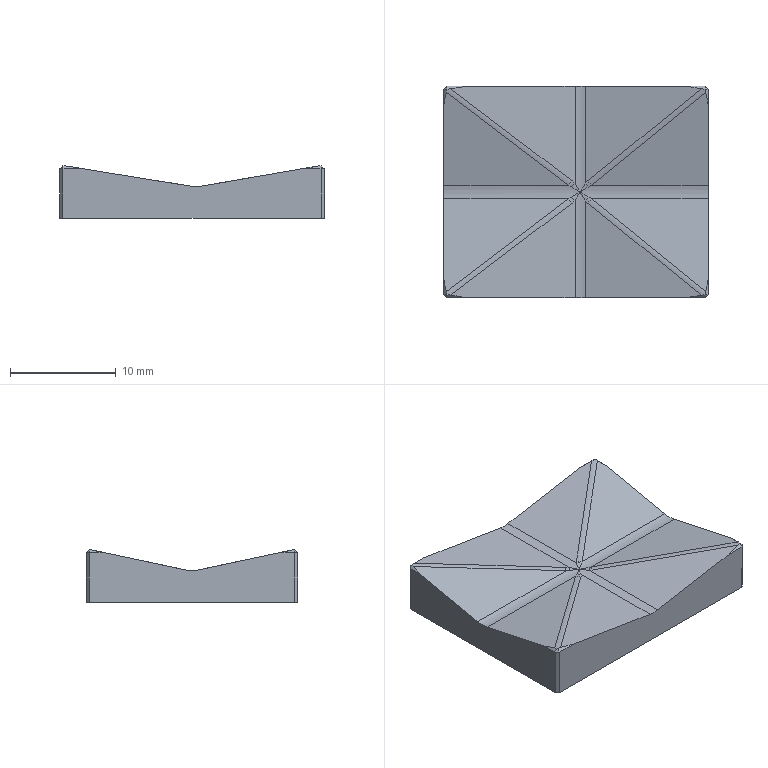Part | SolidWorks | features ICE 2, Chamfer 1, Extrusion 1, Fillet 1 | 1 solid | 42 faces | box 25 x 20 x 4.984 mm | volume 1824 mm3 | plane 29 | cylinder 7 | spline 6 | commonest cylinder face diameters 4 x4 6 x3